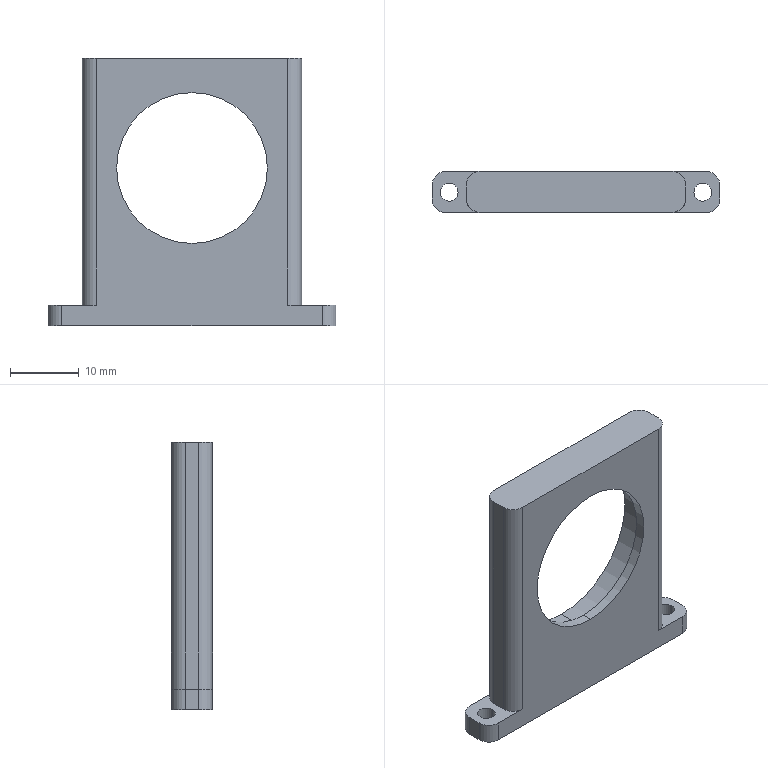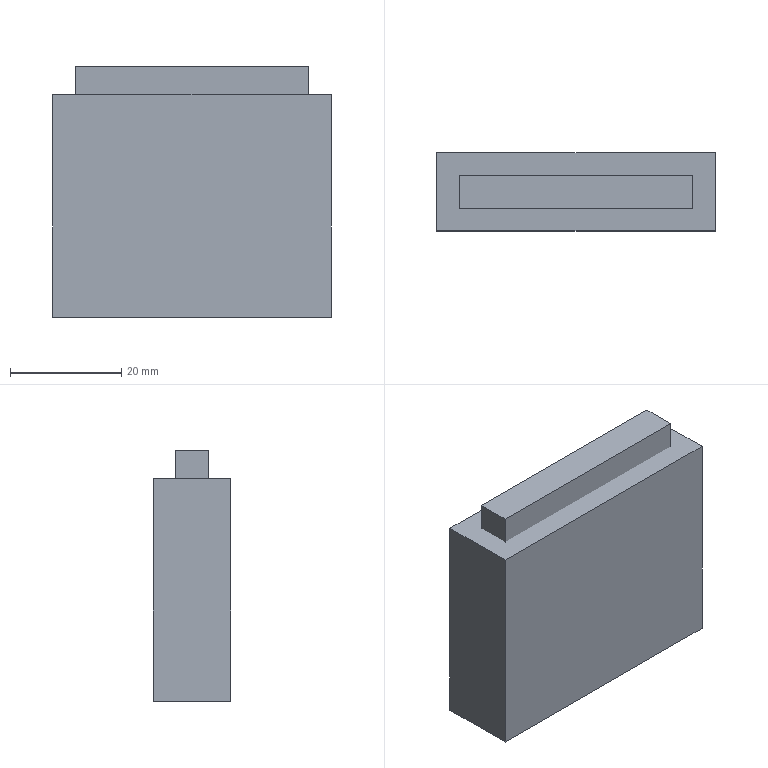CAM job | NX | 3+2 milling, drilling | part box 42 x 6 x 39 mm | stock box 50 x 14 x 45 mm
Tools:
number,name,description,diameter,corner_radius,flute_length,length,flutes
15,D10,Milling Tool-5 Parameters,10.0,0.0,50.0,75.0,2
14,D10JING,Milling Tool-5 Parameters,10.0,0.0,50.0,75.0,2
1,D6A45,Milling Tool-5 Parameters,6.0,0.0,50.0,75.0,2
3,3.3ZT,Drilling Tool,3.3,0.0,35.0,50.0,2
17,2.6ZT,Drilling Tool,2.6,0.0,35.0,50.0,2
Operations:
program,operation,operation_type,tool,method,geometry_group,spindle_rpm,surface_speed,feed_per_tooth,feed_cut,feed_plunge,cut_length_mm,path_length_mm,cut_time_min,machine_time_min
1,FLOOR_WALL_COPY,VolumeBased25DMillingOperation,D10JING,METHOD,A,6500.0,1633.0,0.1154,1500.0,100.0,76.0,130.0,0.0507,0.0561
1,ADAPTIVE_MILLING,CavityMilling,D10,METHOD,A,9500.0,298.0,0.1579,3000.0,1000.0,666.899,760.899,0.2243,0.2337
1,ADAPTIVE_MILLING_COPY,CavityMilling,D10,METHOD,A,9500.0,298.0,0.1579,3000.0,1000.0,666.933,792.633,0.2243,0.2369
1,ADAPTIVE_MILLING_COPY_COPY,CavityMilling,D10,METHOD,A,9500.0,298.0,0.1579,3000.0,1000.0,530.218,662.218,0.1787,0.1919
1,ZLEVEL_PROFILE_COPY_1_COPY_COPY_1_COPY,ZLevelMilling,D10JING,METHOD,A,9500.0,298.0,0.0632,1200.0,1000.0,222.732,450.112,0.1868,0.2095
1,ZLEVEL_PROFILE_COPY_1_COPY_COPY_1_COPY_COPY,ZLevelMilling,D10JING,METHOD,A,9500.0,298.0,0.0632,1200.0,1000.0,131.366,267.366,0.1101,0.1237
1,PLANAR_MILL_COPY_COPY_COPY_COPY_COPY_COPY_1_COPY_1,PlanarMilling,D6A45,METHOD,A,9500.0,179.0,0.0658,1250.0,100.0,84.304,143.304,0.0674,0.0733
1,刀补14,ZLevelMilling,D10JING,METHOD,A,9500.0,298.0,0.0632,1200.0,1000.0,223.132,450.58,0.1872,0.2099
2,FLOOR_WALL_COPY_COPY,VolumeBased25DMillingOperation,D10JING,METHOD,B,6500.0,1633.0,0.1154,1500.0,100.0,408.0,1012.001,0.272,0.3324
2,DRILLING_COPY_1_COPY,Operation,D6A45,METHOD,B,5000.0,94.0,0.035,350.0,0.0,12.0,145.863,0.0343,0.0477
2,DRILLING_COPY_1_COPY_1_1_COPY_1,Operation,3.3ZT,METHOD,B,2000.0,34.0,0.05,200.0,0.0,11.0,82.0,0.055,0.0621
2,DRILLING_COPY_1_COPY_1_1_COPY_1_COPY,Operation,2.6ZT,METHOD,B,2000.0,34.0,0.05,200.0,0.0,16.562,133.246,0.0828,0.0945
2,PLANAR_MILL_COPY_COPY_COPY_COPY_COPY_COPY_1_COPY_1_COPY,PlanarMilling,D6A45,METHOD,B,9500.0,179.0,0.0658,1250.0,100.0,126.453,404.339,0.1012,0.129
3,HOLE_MILLING,CylinderMilling,D10JING,METHOD,C,9500.0,298.0,0.0658,1250.0,100.0,591.758,660.758,0.4734,0.4803
3,HOLE_MILLING_COPY,CylinderMilling,D10JING,METHOD,C,9500.0,298.0,0.0658,1250.0,100.0,226.258,298.258,0.181,0.1882
3,PLANAR_MILL_COPY_COPY_COPY_COPY_COPY_COPY_1_COPY_1_COPY_COPY,PlanarMilling,D6A45,METHOD,C,9500.0,179.0,0.0658,1250.0,100.0,82.378,141.378,0.0659,0.0718